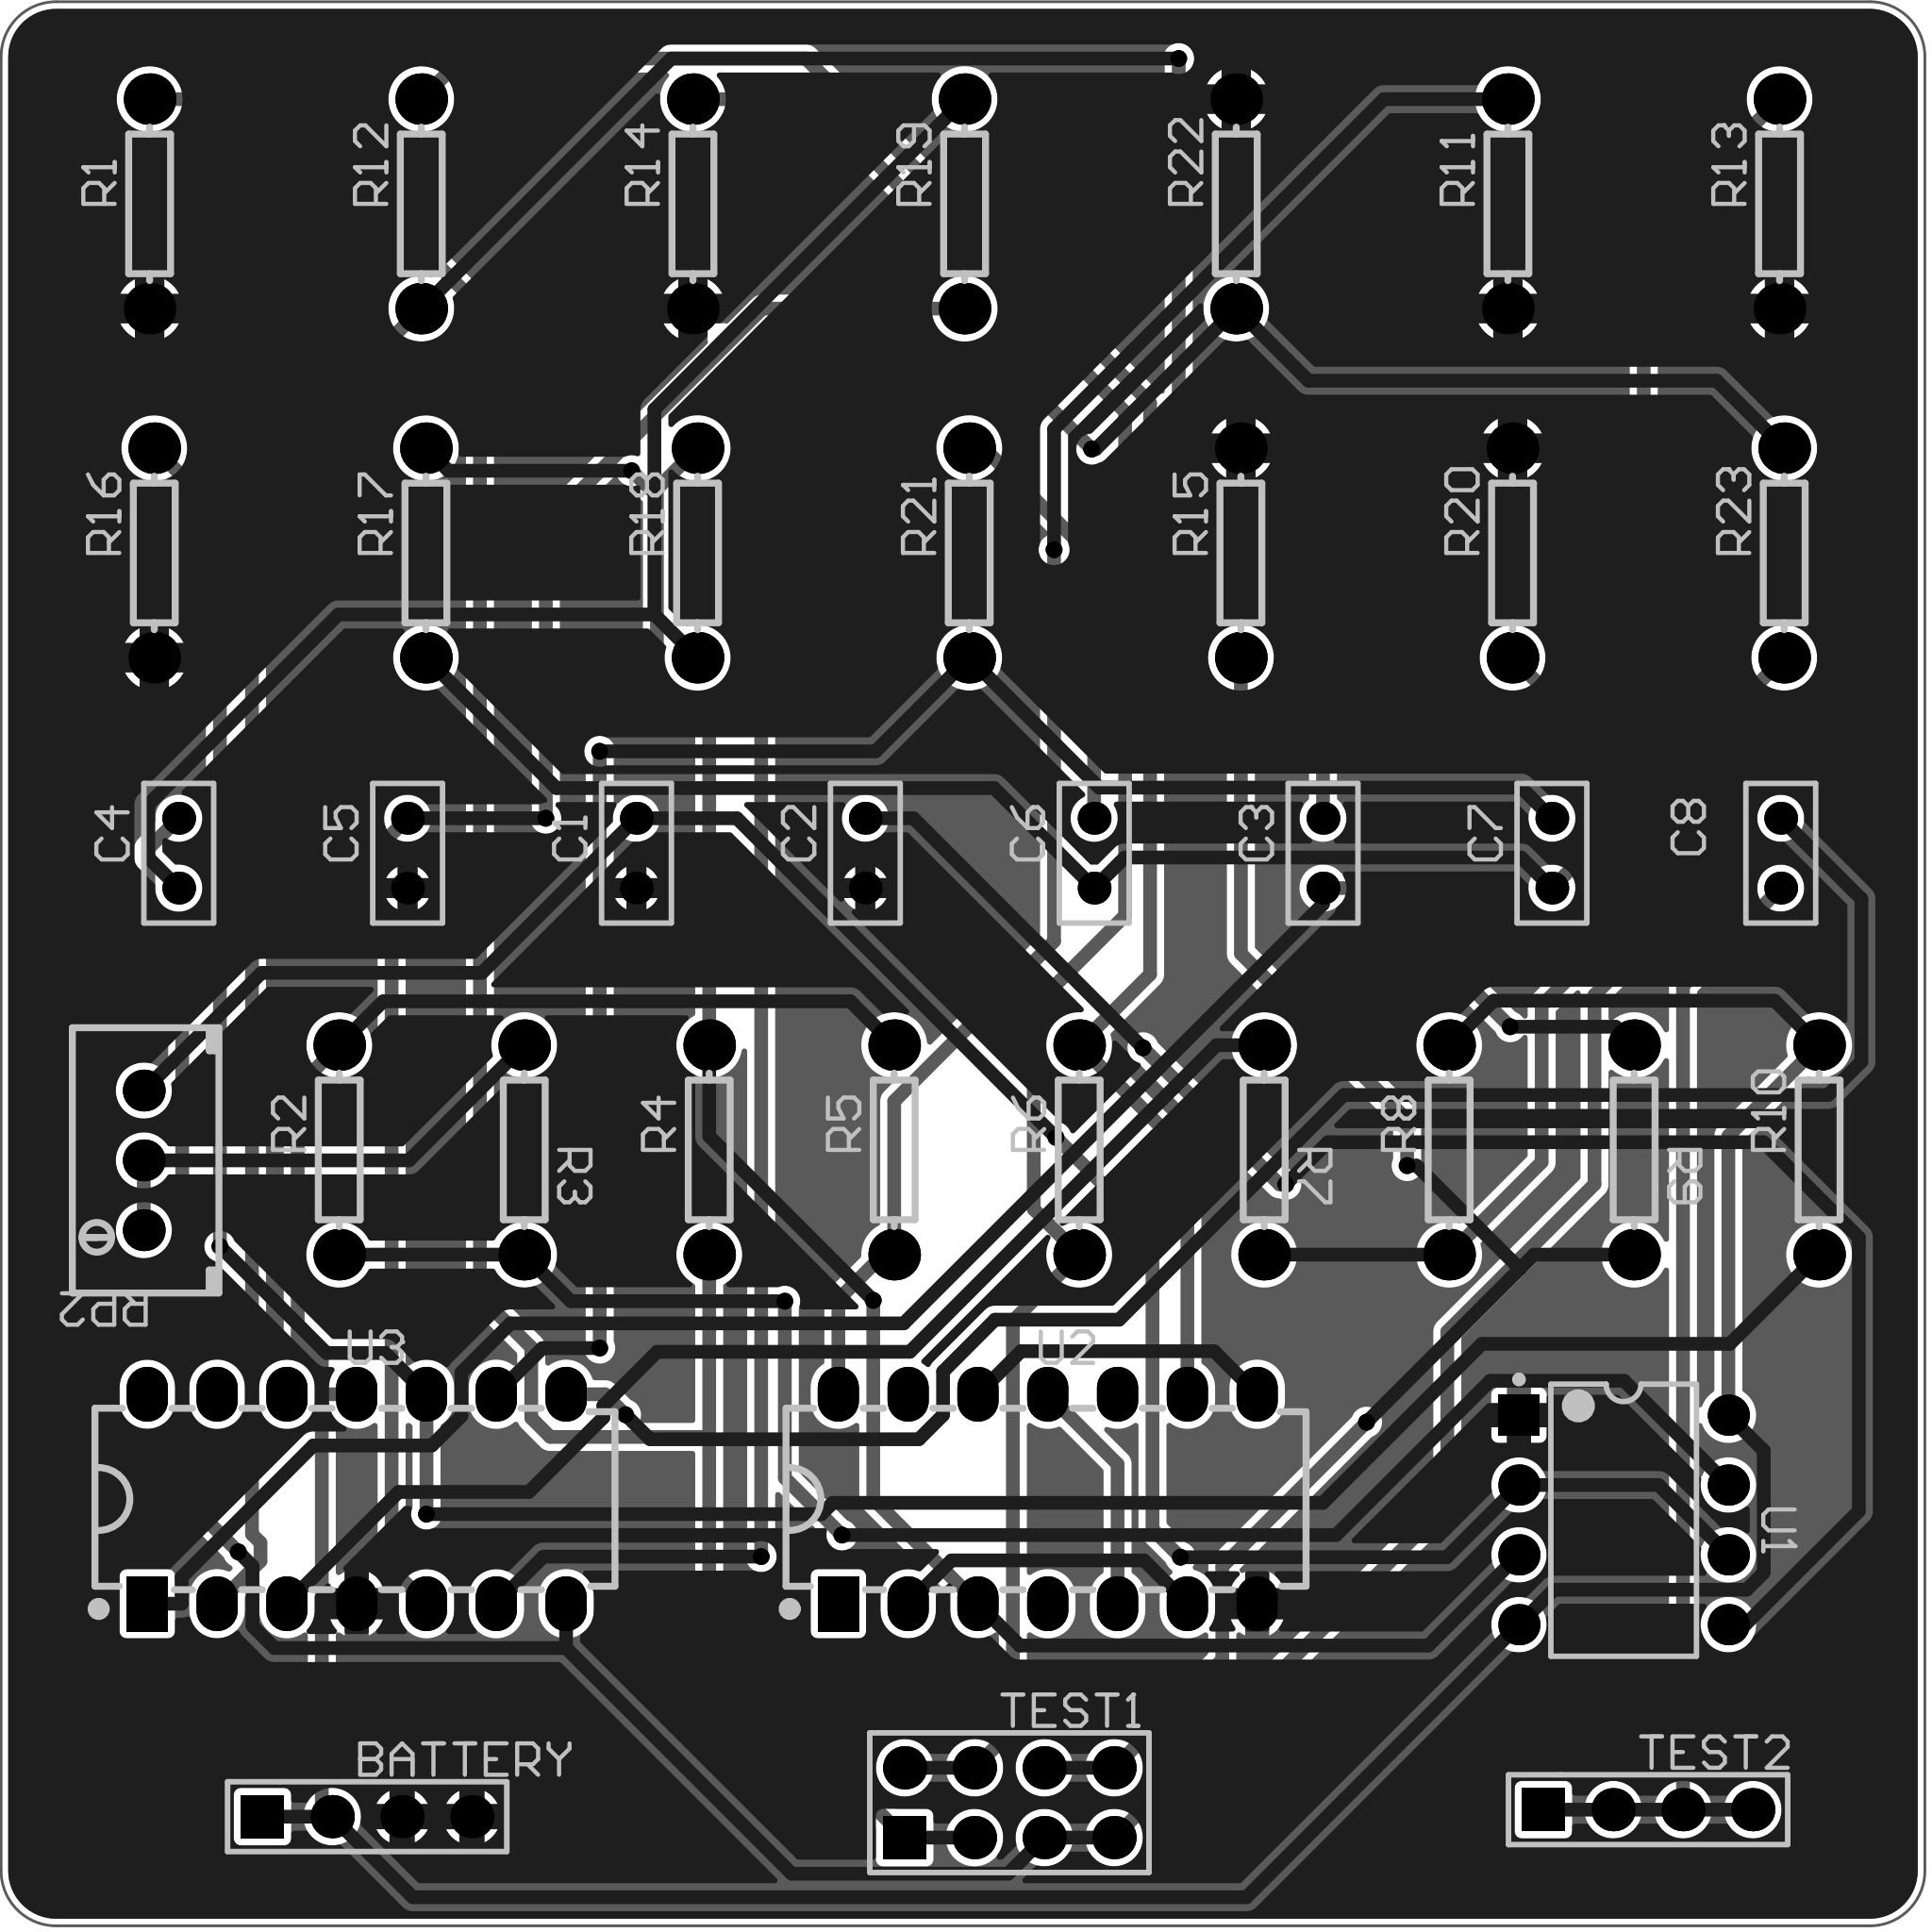Circuit board layout | Altium Designer
Layer stack:
# Altium Designer layer stack of  (unit mm; dielectric type: 0 none, 1 core, 2 prepreg, 3 surface material)
index,name,kind,layer,copper_thickness_mm,dielectric_type,dielectric_thickness_mm,dielectric_material,dielectric_constant
0,Top Silkscreen Layer,other,,,,,,
1,Top Paste Mask Layer,other,,,,,,
2,Top Solder Mask Layer,dielectric,,,3,0,,0
3,Top Layer,copper,Top Layer,0,,,,
4,Substrate-1,dielectric,,,3,0,,0
5,Bottom Layer,copper,Bottom Layer,0,,,,
6,Bottom Solder Mask Layer,dielectric,,,3,0,,0
7,Bottom Paste Mask Layer,other,,,,,,
8,Bottom Silkscreen Layer,other,,,,,,
# drill layer pairs: low layer,high layer
drill_pair,Top Layer,Bottom Layer
Part placement:
Designator,Comment,Layer,Footprint,Center-X(mm),Center-Y(mm),Rotation
R1,60,TopLayer,R_AXIAL-0.3,90.001,146.431,90
R11,1k,TopLayer,R_AXIAL-0.3,139.425,146.431,90
R12,1800,TopLayer,R_AXIAL-0.3,99.885,146.431,90
R13,100,TopLayer,R_AXIAL-0.3,149.31,146.431,90
R14,120,TopLayer,R_AXIAL-0.3,109.77,146.431,90
R15,200,TopLayer,R_AXIAL-0.3,129.709,133.731,90
R16,1350,TopLayer,R_AXIAL-0.3,90.17,133.731,90
R17,41k,TopLayer,R_AXIAL-0.3,100.055,133.731,90
R18,10k,TopLayer,R_AXIAL-0.3,109.94,133.731,90
R19,16500,TopLayer,R_AXIAL-0.3,119.655,146.431,90
R20,50,TopLayer,R_AXIAL-0.3,139.594,133.731,90
R21,90k,TopLayer,R_AXIAL-0.3,119.825,133.731,90
R22,3600,TopLayer,R_AXIAL-0.3,129.54,146.431,90
R23,720,TopLayer,R_AXIAL-0.3,149.479,133.731,90
R4,540,TopLayer,R_AXIAL-0.3,110.363,112.014,90
R6,480,TopLayer,R_AXIAL-0.3,123.825,112.014,90
R9,400,TopLayer,R_AXIAL-0.3,144.018,112.014,270
BATTERY,HDR-M-2.54_1x4,TopLayer,HDR-M-2.54_1X4,97.917,87.757,0
TEST2,test,TopLayer,HDR-M-2.54_1X4,144.526,88.011,0
C1,1n,TopLayer,RAD-0.1,107.714,122.809,90
C2,0.01u,TopLayer,RAD-0.1,116.042,122.809,90
C3,10n,TopLayer,RAD-0.1,132.697,122.809,90
C4,1n,TopLayer,RAD-0.1,91.059,122.809,90
C5,1n,TopLayer,RAD-0.1,99.386,122.809,90
C6,0.1n,TopLayer,RAD-0.1,124.369,122.809,90
C7,0.1n,TopLayer,RAD-0.1,141.024,122.809,90
C8,1n,TopLayer,RAD-0.1,149.352,122.809,90
R2,510,TopLayer,R_AXIAL-0.3,96.901,112.014,90
R3,12k,TopLayer,R_AXIAL-0.3,103.632,112.014,270
R5,1k,TopLayer,R_AXIAL-0.3,117.094,112.014,90
R7,1k,TopLayer,R_AXIAL-0.3,130.556,112.014,270
R8,300,TopLayer,R_AXIAL-0.3,137.287,112.014,90
R10,1k,TopLayer,R_AXIAL-0.3,150.749,112.014,90
RP2,R_3296W_US,TopLayer,RES-ADJ-TH_3296W,89.789,111.633,180
TEST1,test,TopLayer,HDR-M-2.54_2X4,121.285,88.265,0
U1,100kHz,TopLayer,DIP-8_L9.8-W6.6-P2.54-LS7.6-BL,143.637,98.552,270
U2,SN74LS74N,TopLayer,DIP-14_L19.1-W6.4-P2.54-LS7.6-BL,122.682,99.314,0
U3,LM324_C5157701,TopLayer,DIP-14_L18.9-W6.4-P2.54-LS7.6-BL,97.536,99.314,0
Pad and via stacks:
# Altium Designer via and pad stacks of  (unit mm). Each distinct definition once, with the count of objects using it.
# via: kind,start_layer,end_layer,hole_mm,diameter_mm,mode(0 simple;1 top-mid-bottom;2 full stack),diameter_per_layer,count,example_net
# pad: kind,layer,hole_mm,hole_type(0 round;1 square;2 slot),plating,top_size,top_shape(1 round;2 rect;3 octagon;9 rounded rect),mid_size,bottom_size,mode,footprint,size_per_layer,count,example
pad,Multi-Layer,0.8992,0,plated,1.88x1.88,1,1.88x1.88,1.88x1.88,0,R_AXIAL-0.3,,46,R1.1
pad,Multi-Layer,0.889,0,plated,1.575x1.575,2,1.575x1.575,1.575x1.575,0,HDR-M-2.54_1X4,,2,BATTERY.1
pad,Multi-Layer,0.889,0,plated,1.575x1.575,1,1.575x1.575,1.575x1.575,0,HDR-M-2.54_1X4,,6,BATTERY.2
pad,Multi-Layer,0.7112,0,plated,1.194x1.194,1,1.194x1.194,1.194x1.194,0,RAD-0.1,,16,C1.1
pad,Multi-Layer,0.762,0,plated,1.524x1.524,1,1.524x1.524,1.524x1.524,0,RES-ADJ-TH_3296W,,3,RP2.2
pad,Multi-Layer,0.889,0,plated,1.575x1.575,2,1.575x1.575,1.575x1.575,0,HDR-M-2.54_2X4,,1,TEST1.1
pad,Multi-Layer,0.889,0,plated,1.575x1.575,1,1.575x1.575,1.575x1.575,0,HDR-M-2.54_2X4,,7,TEST1.2
pad,Multi-Layer,0.9,0,plated,1.5x1.5,2,1.5x1.5,1.5x1.5,0,DIP-8_L9.8-W6.6-P2.54-LS7.6-BL,,1,U1.1
pad,Multi-Layer,0.9,0,plated,1.5x1.5,1,1.5x1.5,1.5x1.5,0,DIP-8_L9.8-W6.6-P2.54-LS7.6-BL,,7,U1.2
pad,Multi-Layer,1,0,plated,2x1.5,1,2x1.5,2x1.5,0,DIP-14_L19.1-W6.4-P2.54-LS7.6-BL,,13,U2.8
pad,Multi-Layer,1,0,plated,2x1.5,2,2x1.5,2x1.5,0,DIP-14_L19.1-W6.4-P2.54-LS7.6-BL,,1,U2.1
pad,Multi-Layer,1,0,plated,2x1.5,1,2x1.5,2x1.5,0,DIP-14_L18.9-W6.4-P2.54-LS7.6-BL,,13,U3.8
pad,Multi-Layer,1,0,plated,2x1.5,2,2x1.5,2x1.5,0,DIP-14_L18.9-W6.4-P2.54-LS7.6-BL,,1,U3.1
via,Top Layer,Bottom Layer,0.3048,0.61,0,,22,TEST1_5
Copper pours:
name,layer,net,type(0 solid;1 hatched;2 none)
Top Layer-GND,Top Layer,GND,0
Bottom Layer-GND,Bottom Layer,GND,0
Design rules, without the lines most boards share:
# Altium Designer design rules of  (exported by Altium Designer, unit mm)
# columns: name | kind | enabled | priority | scope1 | scope2 | descriptor | typed fields (field=value)
HoleToHoleClearance | 52 | enabled | 1 | All | All | Hole To Hole Clearance (Gap=10mil) (All),(All) | gap=0.254
DiffPairsRouting | 51 | enabled | 1 | All | All | Differential Pairs Uncoupled Length using the Gap Constraints (Min=10mil) (Max=10mil) (Prefered=10mil)  and Width Constraints (Min=15mil) (Max=15mil) (Prefered=15mil) (All) |
Plane_Default | 0 | disabled | 1 | All | All | Clearance Constraint (Gap=9.843mil) (Disabled)(All),(All) | gap=0.25
Plane_Default_1 | 63 | disabled | 1 | All | All | Board Clearance Constraint (Gap=0mil) (Disabled)(All) |
Copper_Default | 0 | disabled | 2 | All | All | Clearance Constraint (Gap=9.843mil) (Disabled)(All),(All) | gap=0.25
Copper_Default_1 | 63 | disabled | 2 | All | All | Board Clearance Constraint (Gap=0mil) (Disabled)(All) |
Copper_gge9694 | 0 | disabled | 3 | All | All | Clearance Constraint (Gap=9.843mil) (Disabled)(All),(All) | gap=0.25
Copper_gge9694_1 | 63 | disabled | 3 | All | All | Board Clearance Constraint (Gap=0mil) (Disabled)(All) |
Copper_gge9712 | 0 | disabled | 4 | All | All | Clearance Constraint (Gap=9.843mil) (Disabled)(All),(All) | gap=0.25
Copper_gge9712_1 | 63 | disabled | 4 | All | All | Board Clearance Constraint (Gap=0mil) (Disabled)(All) |
Default | 0 | enabled | 5 | All | All | Clearance Constraint (Gap=9.843mil) (All),(All) | gap=0.25
Default_1 | 63 | enabled | 5 | All | All | Board Clearance Constraint (Gap=0mil) (All) |
Default_2 | 2 | enabled | 1 | All | All | Width Constraint (Min=19.7mil) (Max=1000mil) (Preferred=19.7mil) (All) |
Default_3 | 11 | enabled | 1 | All | All | Routing Via (MinHoleWidth=12.008mil) (MaxHoleWidth=2362mil) (PreferredHoleWidth=12.008mil) (MinWidth=24.016mil) (MaxWidth=3938mil) (PreferedWidth=24.016mil) (All) | via_min_hole=0.305 via_max_hole=59.995 via_preferred_diameter=0.61 via_preferred_hole=0.305
Default_4 | 6 | enabled | 1 | All | All | Power Plane Connect Rule(Relief Connect )(Expansion=20mil) (Conductor Width=0mil) (Air Gap=10mil) (Entries=4) (All) | relief_conductor_width=0 relief_entries=4 relief_expansion=0.508
gge9694 | 20 | disabled | 1 | All | All | Polygon Connect Rule(Relief Connect )(Conductor Width=0mil) (Relief Angle=90 Angle) (Entries=4) (Air Gap Width=10mil) (Disabled)(All),(All) | connect_style(0=relief,1=direct,2=none)=0 relief_conductor_width=0 relief_entries=4
gge9712 | 20 | disabled | 2 | All | All | Polygon Connect Rule(Relief Connect )(Conductor Width=0mil) (Relief Angle=90 Angle) (Entries=4) (Air Gap Width=10mil) (Disabled)(All),(All) | connect_style(0=relief,1=direct,2=none)=0 relief_conductor_width=0 relief_entries=4
Default_5 | 20 | enabled | 3 | All | All | Polygon Connect Rule(Relief Connect )(Conductor Width=0mil) (Relief Angle=90 Angle) (Entries=4) (Air Gap Width=10mil) (All),(All) | connect_style(0=relief,1=direct,2=none)=0 relief_conductor_width=0 relief_entries=4
Common | 14 | enabled | 1 | All | All | Paste Mask Expansion (Expansion =0mil) (All) | expansion=0
Common_1 | 13 | enabled | 2 | All | All | Solder Mask Expansion (Expansion =2mil) (All) | expansion=0.0508
Common_2 | 13 | enabled | 1 | IsVia | All | Solder Mask Expansion (Expansion =-1000mil) (IsVia) | expansion=-25.4